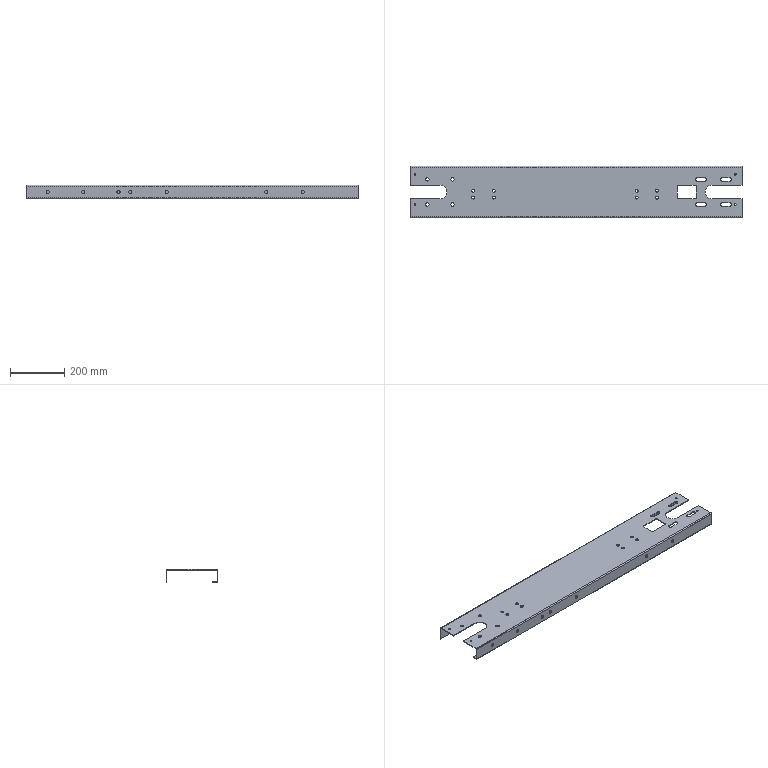Part | STEP file | PN_0037_side beam | 1 solid | 101 faces | box 1220 x 190 x 50 mm | volume 1029642 mm3 | cylinder 71 | plane 30 | commonest cylinder face diameters 12 x34 11 x16 7 x8 10 x4 1.473 x3 7.473 x3